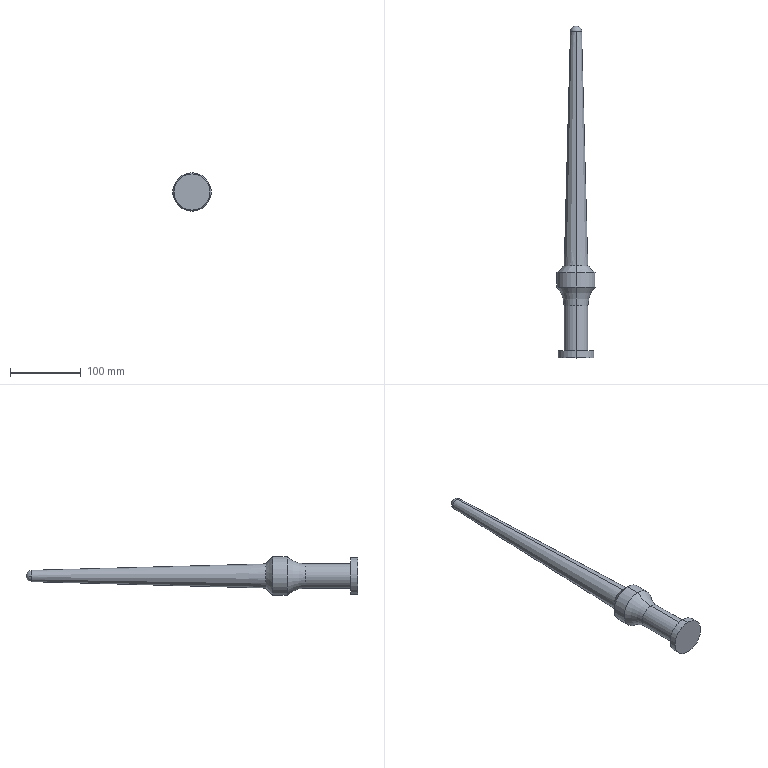Part | SolidWorks | features Revolution 1 | 1 solid | 16 faces | box 54 x 468 x 54 mm | volume 343926 mm3 | cylinder 6 | cone 4 | torus 2 | sphere 2 | plane 2 | commonest cylinder face diameters 34 x2 51 x2 54 x2
STEP:
#1=CARTESIAN_POINT('',(0.,0.,25.5));
#2=VERTEX_POINT('',#1);
#3=CARTESIAN_POINT('',(0.,0.,-25.5));
#4=VERTEX_POINT('',#3);
#5=CARTESIAN_POINT('',(0.,0.,0.));
#6=DIRECTION('',(0.,1.,0.));
#7=DIRECTION('',(0.,0.,1.));
#8=AXIS2_PLACEMENT_3D('',#5,#6,#7);
#9=CIRCLE('',#8,25.5);
#10=EDGE_CURVE('',#2,#4,#9,.T.);
#11=ORIENTED_EDGE('',*,*,#10,.T.);
#12=CARTESIAN_POINT('',(0.,10.,-25.5));
#13=VERTEX_POINT('',#12);
#14=CARTESIAN_POINT('',(0.,0.,-25.5));
#15=DIRECTION('',(0.,1.,0.));
#16=VECTOR('',#15,1000.);
#17=LINE('',#14,#16);
#18=EDGE_CURVE('',#4,#13,#17,.T.);
#19=ORIENTED_EDGE('',*,*,#18,.T.);
#20=CARTESIAN_POINT('',(0.,10.,25.5));
#21=VERTEX_POINT('',#20);
#22=CARTESIAN_POINT('',(0.,10.,0.));
#23=DIRECTION('',(0.,1.,0.));
#24=DIRECTION('',(0.,0.,1.));
#25=AXIS2_PLACEMENT_3D('',#22,#23,#24);
#26=CIRCLE('',#25,25.5);
#27=EDGE_CURVE('',#21,#13,#26,.T.);
#28=ORIENTED_EDGE('',*,*,#27,.F.);
#29=CARTESIAN_POINT('',(0.,0.,25.5));
#30=DIRECTION('',(0.,1.,0.));
#31=VECTOR('',#30,1000.);
#32=LINE('',#29,#31);
#33=EDGE_CURVE('',#2,#21,#32,.T.);
#34=ORIENTED_EDGE('',*,*,#33,.F.);
#35=EDGE_LOOP('',(#11,#19,#28,#34));
#36=FACE_OUTER_BOUND('',#35,.T.);
#37=CARTESIAN_POINT('',(0.,0.,0.));
#38=DIRECTION('',(0.,1.,0.));
#39=DIRECTION('',(0.,0.,1.));
#40=AXIS2_PLACEMENT_3D('',#37,#38,#39);
#41=CYLINDRICAL_SURFACE('',#40,25.5);
#42=ADVANCED_FACE('',(#36),#41,.T.);
#43=CARTESIAN_POINT('',(0.,10.,17.));
#44=VERTEX_POINT('',#43);
#45=CARTESIAN_POINT('',(0.,10.,-17.));
#46=VERTEX_POINT('',#45);
#47=CARTESIAN_POINT('',(0.,10.,0.));
#48=DIRECTION('',(0.,1.,0.));
#49=DIRECTION('',(0.,0.,1.));
#50=AXIS2_PLACEMENT_3D('',#47,#48,#49);
#51=CIRCLE('',#50,17.);
#52=EDGE_CURVE('',#44,#46,#51,.T.);
#53=ORIENTED_EDGE('',*,*,#52,.T.);
#54=CARTESIAN_POINT('',(0.,73.542,-17.));
#55=VERTEX_POINT('',#54);
#56=CARTESIAN_POINT('',(0.,0.,-17.));
#57=DIRECTION('',(0.,1.,0.));
#58=VECTOR('',#57,1000.);
#59=LINE('',#56,#58);
#60=EDGE_CURVE('',#46,#55,#59,.T.);
#61=ORIENTED_EDGE('',*,*,#60,.T.);
#62=CARTESIAN_POINT('',(0.,73.542,17.));
#63=VERTEX_POINT('',#62);
#64=CARTESIAN_POINT('',(0.,73.542,0.));
#65=DIRECTION('',(0.,1.,0.));
#66=DIRECTION('',(0.,0.,1.));
#67=AXIS2_PLACEMENT_3D('',#64,#65,#66);
#68=CIRCLE('',#67,17.);
#69=EDGE_CURVE('',#63,#55,#68,.T.);
#70=ORIENTED_EDGE('',*,*,#69,.F.);
#71=CARTESIAN_POINT('',(0.,0.,17.));
#72=DIRECTION('',(0.,1.,0.));
#73=VECTOR('',#72,1000.);
#74=LINE('',#71,#73);
#75=EDGE_CURVE('',#44,#63,#74,.T.);
#76=ORIENTED_EDGE('',*,*,#75,.F.);
#77=EDGE_LOOP('',(#53,#61,#70,#76));
#78=FACE_OUTER_BOUND('',#77,.T.);
#79=CARTESIAN_POINT('',(0.,0.,0.));
#80=DIRECTION('',(0.,1.,0.));
#81=DIRECTION('',(0.,0.,1.));
#82=AXIS2_PLACEMENT_3D('',#79,#80,#81);
#83=CYLINDRICAL_SURFACE('',#82,17.);
#84=ADVANCED_FACE('',(#78),#83,.T.);
#85=CARTESIAN_POINT('',(0.,100.,-27.));
#86=VERTEX_POINT('',#85);
#87=CARTESIAN_POINT('',(0.,100.,27.));
#88=VERTEX_POINT('',#87);
#89=CARTESIAN_POINT('',(0.,100.,0.));
#90=DIRECTION('',(0.,1.,0.));
#91=DIRECTION('',(0.,0.,1.));
#92=AXIS2_PLACEMENT_3D('',#89,#90,#91);
#93=CIRCLE('',#92,27.);
#94=EDGE_CURVE('',#86,#88,#93,.T.);
#95=ORIENTED_EDGE('',*,*,#94,.F.);
#96=CARTESIAN_POINT('',(0.,73.542,-57.));
#97=DIRECTION('',(1.,0.,0.));
#98=DIRECTION('',(0.,0.,-1.));
#99=AXIS2_PLACEMENT_3D('',#96,#97,#98);
#100=CIRCLE('',#99,40.);
#101=EDGE_CURVE('',#86,#55,#100,.T.);
#102=ORIENTED_EDGE('',*,*,#101,.T.);
#103=CARTESIAN_POINT('',(0.,73.542,0.));
#104=DIRECTION('',(0.,1.,0.));
#105=DIRECTION('',(0.,0.,1.));
#106=AXIS2_PLACEMENT_3D('',#103,#104,#105);
#107=CIRCLE('',#106,17.);
#108=EDGE_CURVE('',#55,#63,#107,.T.);
#109=ORIENTED_EDGE('',*,*,#108,.T.);
#110=CARTESIAN_POINT('',(0.,73.542,57.));
#111=DIRECTION('',(-1.,0.,0.));
#112=DIRECTION('',(0.,0.,1.));
#113=AXIS2_PLACEMENT_3D('',#110,#111,#112);
#114=CIRCLE('',#113,40.);
#115=EDGE_CURVE('',#88,#63,#114,.T.);
#116=ORIENTED_EDGE('',*,*,#115,.F.);
#117=EDGE_LOOP('',(#95,#102,#109,#116));
#118=FACE_OUTER_BOUND('',#117,.T.);
#119=CARTESIAN_POINT('',(0.,73.542,0.));
#120=DIRECTION('',(0.,1.,0.));
#121=DIRECTION('',(0.,0.,1.));
#122=AXIS2_PLACEMENT_3D('',#119,#120,#121);
#123=TOROIDAL_SURFACE('',#122,57.,40.);
#124=ADVANCED_FACE('',(#118),#123,.F.);
#125=CARTESIAN_POINT('',(0.,100.,0.));
#126=DIRECTION('',(0.,1.,0.));
#127=DIRECTION('',(0.,0.,1.));
#128=AXIS2_PLACEMENT_3D('',#125,#126,#127);
#129=CIRCLE('',#128,27.);
#130=EDGE_CURVE('',#88,#86,#129,.T.);
#131=ORIENTED_EDGE('',*,*,#130,.T.);
#132=CARTESIAN_POINT('',(0.,120.,-27.));
#133=VERTEX_POINT('',#132);
#134=CARTESIAN_POINT('',(0.,0.,-27.));
#135=DIRECTION('',(0.,1.,0.));
#136=VECTOR('',#135,1000.);
#137=LINE('',#134,#136);
#138=EDGE_CURVE('',#86,#133,#137,.T.);
#139=ORIENTED_EDGE('',*,*,#138,.T.);
#140=CARTESIAN_POINT('',(0.,120.,27.));
#141=VERTEX_POINT('',#140);
#142=CARTESIAN_POINT('',(0.,120.,0.));
#143=DIRECTION('',(0.,1.,0.));
#144=DIRECTION('',(0.,0.,1.));
#145=AXIS2_PLACEMENT_3D('',#142,#143,#144);
#146=CIRCLE('',#145,27.);
#147=EDGE_CURVE('',#141,#133,#146,.T.);
#148=ORIENTED_EDGE('',*,*,#147,.F.);
#149=CARTESIAN_POINT('',(0.,0.,27.));
#150=DIRECTION('',(0.,1.,0.));
#151=VECTOR('',#150,1000.);
#152=LINE('',#149,#151);
#153=EDGE_CURVE('',#88,#141,#152,.T.);
#154=ORIENTED_EDGE('',*,*,#153,.F.);
#155=EDGE_LOOP('',(#131,#139,#148,#154));
#156=FACE_OUTER_BOUND('',#155,.T.);
#157=CARTESIAN_POINT('',(0.,0.,0.));
#158=DIRECTION('',(0.,1.,0.));
#159=DIRECTION('',(0.,0.,1.));
#160=AXIS2_PLACEMENT_3D('',#157,#158,#159);
#161=CYLINDRICAL_SURFACE('',#160,27.);
#162=ADVANCED_FACE('',(#156),#161,.T.);
#163=CARTESIAN_POINT('',(0.,130.,17.));
#164=VERTEX_POINT('',#163);
#165=CARTESIAN_POINT('',(0.,130.,-17.));
#166=VERTEX_POINT('',#165);
#167=CARTESIAN_POINT('',(0.,130.,0.));
#168=DIRECTION('',(0.,1.,0.));
#169=DIRECTION('',(0.,0.,1.));
#170=AXIS2_PLACEMENT_3D('',#167,#168,#169);
#171=CIRCLE('',#170,17.);
#172=EDGE_CURVE('',#164,#166,#171,.T.);
#173=ORIENTED_EDGE('',*,*,#172,.F.);
#174=CARTESIAN_POINT('',(0.,120.,27.));
#175=DIRECTION('',(0.,-0.7071,0.7071));
#176=VECTOR('',#175,1000.);
#177=LINE('',#174,#176);
#178=EDGE_CURVE('',#164,#141,#177,.T.);
#179=ORIENTED_EDGE('',*,*,#178,.T.);
#180=ORIENTED_EDGE('',*,*,#147,.T.);
#181=CARTESIAN_POINT('',(0.,120.,-27.));
#182=DIRECTION('',(0.,-0.7071,-0.7071));
#183=VECTOR('',#182,1000.);
#184=LINE('',#181,#183);
#185=EDGE_CURVE('',#166,#133,#184,.T.);
#186=ORIENTED_EDGE('',*,*,#185,.F.);
#187=EDGE_LOOP('',(#173,#179,#180,#186));
#188=FACE_OUTER_BOUND('',#187,.T.);
#189=CARTESIAN_POINT('',(0.,120.,0.));
#190=DIRECTION('',(0.,-1.,0.));
#191=DIRECTION('',(0.,0.,-1.));
#192=AXIS2_PLACEMENT_3D('',#189,#190,#191);
#193=CONICAL_SURFACE('',#192,27.,0.7854);
#194=ADVANCED_FACE('',(#188),#193,.T.);
#195=CARTESIAN_POINT('',(0.,460.218,7.997));
#196=VERTEX_POINT('',#195);
#197=CARTESIAN_POINT('',(7.997,460.218,0.));
#198=VERTEX_POINT('',#197);
#199=CARTESIAN_POINT('',(0.,460.218,0.));
#200=DIRECTION('',(0.,1.,0.));
#201=DIRECTION('',(0.,0.,1.));
#202=AXIS2_PLACEMENT_3D('',#199,#200,#201);
#203=CIRCLE('',#202,7.997);
#204=EDGE_CURVE('',#196,#198,#203,.T.);
#205=ORIENTED_EDGE('',*,*,#204,.F.);
#206=CARTESIAN_POINT('',(0.,130.,17.));
#207=DIRECTION('',(0.,-0.9996,0.02725));
#208=VECTOR('',#207,1000.);
#209=LINE('',#206,#208);
#210=EDGE_CURVE('',#196,#164,#209,.T.);
#211=ORIENTED_EDGE('',*,*,#210,.T.);
#212=ORIENTED_EDGE('',*,*,#172,.T.);
#213=CARTESIAN_POINT('',(0.,460.218,-7.997));
#214=VERTEX_POINT('',#213);
#215=CARTESIAN_POINT('',(0.,130.,-17.));
#216=DIRECTION('',(0.,-0.9996,-0.02725));
#217=VECTOR('',#216,1000.);
#218=LINE('',#215,#217);
#219=EDGE_CURVE('',#214,#166,#218,.T.);
#220=ORIENTED_EDGE('',*,*,#219,.F.);
#221=CARTESIAN_POINT('',(0.,460.218,0.));
#222=DIRECTION('',(0.,1.,0.));
#223=DIRECTION('',(0.,0.,1.));
#224=AXIS2_PLACEMENT_3D('',#221,#222,#223);
#225=CIRCLE('',#224,7.997);
#226=EDGE_CURVE('',#198,#214,#225,.T.);
#227=ORIENTED_EDGE('',*,*,#226,.F.);
#228=EDGE_LOOP('',(#205,#211,#212,#220,#227));
#229=FACE_OUTER_BOUND('',#228,.T.);
#230=CARTESIAN_POINT('',(0.,130.,0.));
#231=DIRECTION('',(0.,-1.,0.));
#232=DIRECTION('',(0.,0.,-1.));
#233=AXIS2_PLACEMENT_3D('',#230,#231,#232);
#234=CONICAL_SURFACE('',#233,17.,0.02726);
#235=ADVANCED_FACE('',(#229),#234,.T.);
#236=ORIENTED_EDGE('',*,*,#226,.T.);
#237=CARTESIAN_POINT('',(-7.997,460.218,0.));
#238=VERTEX_POINT('',#237);
#239=CARTESIAN_POINT('',(0.,460.218,0.));
#240=DIRECTION('',(0.,1.,0.));
#241=DIRECTION('',(0.,0.,1.));
#242=AXIS2_PLACEMENT_3D('',#239,#240,#241);
#243=CIRCLE('',#242,7.997);
#244=EDGE_CURVE('',#214,#238,#243,.T.);
#245=ORIENTED_EDGE('',*,*,#244,.T.);
#246=CARTESIAN_POINT('',(0.,468.,0.));
#247=VERTEX_POINT('',#246);
#248=CARTESIAN_POINT('',(0.,460.,0.));
#249=DIRECTION('',(0.,0.,-1.));
#250=DIRECTION('',(-1.,0.,0.));
#251=AXIS2_PLACEMENT_3D('',#248,#249,#250);
#252=CIRCLE('',#251,8.);
#253=EDGE_CURVE('',#238,#247,#252,.T.);
#254=ORIENTED_EDGE('',*,*,#253,.T.);
#255=CARTESIAN_POINT('',(0.,460.,0.));
#256=DIRECTION('',(0.,0.,1.));
#257=DIRECTION('',(1.,0.,0.));
#258=AXIS2_PLACEMENT_3D('',#255,#256,#257);
#259=CIRCLE('',#258,8.);
#260=EDGE_CURVE('',#198,#247,#259,.T.);
#261=ORIENTED_EDGE('',*,*,#260,.F.);
#262=EDGE_LOOP('',(#236,#245,#254,#261));
#263=FACE_OUTER_BOUND('',#262,.T.);
#264=CARTESIAN_POINT('',(0.,460.,0.));
#265=DIRECTION('',(0.,0.,-1.));
#266=DIRECTION('',(1.,0.,0.));
#267=AXIS2_PLACEMENT_3D('',#264,#265,#266);
#268=SPHERICAL_SURFACE('',#267,8.);
#269=ADVANCED_FACE('',(#263),#268,.T.);
#270=ORIENTED_EDGE('',*,*,#253,.F.);
#271=CARTESIAN_POINT('',(0.,460.218,0.));
#272=DIRECTION('',(0.,1.,0.));
#273=DIRECTION('',(0.,0.,1.));
#274=AXIS2_PLACEMENT_3D('',#271,#272,#273);
#275=CIRCLE('',#274,7.997);
#276=EDGE_CURVE('',#238,#196,#275,.T.);
#277=ORIENTED_EDGE('',*,*,#276,.T.);
#278=ORIENTED_EDGE('',*,*,#204,.T.);
#279=ORIENTED_EDGE('',*,*,#260,.T.);
#280=EDGE_LOOP('',(#270,#277,#278,#279));
#281=FACE_OUTER_BOUND('',#280,.T.);
#282=CARTESIAN_POINT('',(0.,460.,0.));
#283=DIRECTION('',(0.,0.,-1.));
#284=DIRECTION('',(1.,0.,0.));
#285=AXIS2_PLACEMENT_3D('',#282,#283,#284);
#286=SPHERICAL_SURFACE('',#285,8.);
#287=ADVANCED_FACE('',(#281),#286,.T.);
#288=ORIENTED_EDGE('',*,*,#210,.F.);
#289=ORIENTED_EDGE('',*,*,#276,.F.);
#290=ORIENTED_EDGE('',*,*,#244,.F.);
#291=ORIENTED_EDGE('',*,*,#219,.T.);
#292=CARTESIAN_POINT('',(0.,130.,0.));
#293=DIRECTION('',(0.,1.,0.));
#294=DIRECTION('',(0.,0.,1.));
#295=AXIS2_PLACEMENT_3D('',#292,#293,#294);
#296=CIRCLE('',#295,17.);
#297=EDGE_CURVE('',#166,#164,#296,.T.);
#298=ORIENTED_EDGE('',*,*,#297,.T.);
#299=EDGE_LOOP('',(#288,#289,#290,#291,#298));
#300=FACE_OUTER_BOUND('',#299,.T.);
#301=CARTESIAN_POINT('',(0.,130.,0.));
#302=DIRECTION('',(0.,-1.,0.));
#303=DIRECTION('',(0.,0.,-1.));
#304=AXIS2_PLACEMENT_3D('',#301,#302,#303);
#305=CONICAL_SURFACE('',#304,17.,0.02726);
#306=ADVANCED_FACE('',(#300),#305,.T.);
#307=ORIENTED_EDGE('',*,*,#178,.F.);
#308=ORIENTED_EDGE('',*,*,#297,.F.);
#309=ORIENTED_EDGE('',*,*,#185,.T.);
#310=CARTESIAN_POINT('',(0.,120.,0.));
#311=DIRECTION('',(0.,1.,0.));
#312=DIRECTION('',(0.,0.,1.));
#313=AXIS2_PLACEMENT_3D('',#310,#311,#312);
#314=CIRCLE('',#313,27.);
#315=EDGE_CURVE('',#133,#141,#314,.T.);
#316=ORIENTED_EDGE('',*,*,#315,.T.);
#317=EDGE_LOOP('',(#307,#308,#309,#316));
#318=FACE_OUTER_BOUND('',#317,.T.);
#319=CARTESIAN_POINT('',(0.,120.,0.));
#320=DIRECTION('',(0.,-1.,0.));
#321=DIRECTION('',(0.,0.,-1.));
#322=AXIS2_PLACEMENT_3D('',#319,#320,#321);
#323=CONICAL_SURFACE('',#322,27.,0.7854);
#324=ADVANCED_FACE('',(#318),#323,.T.);
#325=ORIENTED_EDGE('',*,*,#138,.F.);
#326=ORIENTED_EDGE('',*,*,#94,.T.);
#327=ORIENTED_EDGE('',*,*,#153,.T.);
#328=ORIENTED_EDGE('',*,*,#315,.F.);
#329=EDGE_LOOP('',(#325,#326,#327,#328));
#330=FACE_OUTER_BOUND('',#329,.T.);
#331=CARTESIAN_POINT('',(0.,0.,0.));
#332=DIRECTION('',(0.,1.,0.));
#333=DIRECTION('',(0.,0.,1.));
#334=AXIS2_PLACEMENT_3D('',#331,#332,#333);
#335=CYLINDRICAL_SURFACE('',#334,27.);
#336=ADVANCED_FACE('',(#330),#335,.T.);
#337=ORIENTED_EDGE('',*,*,#101,.F.);
#338=ORIENTED_EDGE('',*,*,#130,.F.);
#339=ORIENTED_EDGE('',*,*,#115,.T.);
#340=ORIENTED_EDGE('',*,*,#69,.T.);
#341=EDGE_LOOP('',(#337,#338,#339,#340));
#342=FACE_OUTER_BOUND('',#341,.T.);
#343=CARTESIAN_POINT('',(0.,73.542,0.));
#344=DIRECTION('',(0.,1.,0.));
#345=DIRECTION('',(0.,0.,1.));
#346=AXIS2_PLACEMENT_3D('',#343,#344,#345);
#347=TOROIDAL_SURFACE('',#346,57.,40.);
#348=ADVANCED_FACE('',(#342),#347,.F.);
#349=ORIENTED_EDGE('',*,*,#60,.F.);
#350=CARTESIAN_POINT('',(0.,10.,0.));
#351=DIRECTION('',(0.,1.,0.));
#352=DIRECTION('',(0.,0.,1.));
#353=AXIS2_PLACEMENT_3D('',#350,#351,#352);
#354=CIRCLE('',#353,17.);
#355=EDGE_CURVE('',#46,#44,#354,.T.);
#356=ORIENTED_EDGE('',*,*,#355,.T.);
#357=ORIENTED_EDGE('',*,*,#75,.T.);
#358=ORIENTED_EDGE('',*,*,#108,.F.);
#359=EDGE_LOOP('',(#349,#356,#357,#358));
#360=FACE_OUTER_BOUND('',#359,.T.);
#361=CARTESIAN_POINT('',(0.,0.,0.));
#362=DIRECTION('',(0.,1.,0.));
#363=DIRECTION('',(0.,0.,1.));
#364=AXIS2_PLACEMENT_3D('',#361,#362,#363);
#365=CYLINDRICAL_SURFACE('',#364,17.);
#366=ADVANCED_FACE('',(#360),#365,.T.);
#367=ORIENTED_EDGE('',*,*,#52,.F.);
#368=ORIENTED_EDGE('',*,*,#355,.F.);
#369=EDGE_LOOP('',(#367,#368));
#370=FACE_BOUND('',#369,.T.);
#371=ORIENTED_EDGE('',*,*,#27,.T.);
#372=CARTESIAN_POINT('',(0.,10.,0.));
#373=DIRECTION('',(0.,1.,0.));
#374=DIRECTION('',(0.,0.,1.));
#375=AXIS2_PLACEMENT_3D('',#372,#373,#374);
#376=CIRCLE('',#375,25.5);
#377=EDGE_CURVE('',#13,#21,#376,.T.);
#378=ORIENTED_EDGE('',*,*,#377,.T.);
#379=EDGE_LOOP('',(#371,#378));
#380=FACE_OUTER_BOUND('',#379,.T.);
#381=CARTESIAN_POINT('',(25.5,10.,0.));
#382=DIRECTION('',(0.,-1.,0.));
#383=DIRECTION('',(0.,0.,-1.));
#384=AXIS2_PLACEMENT_3D('',#381,#382,#383);
#385=PLANE('',#384);
#386=ADVANCED_FACE('',(#370,#380),#385,.F.);
#387=ORIENTED_EDGE('',*,*,#18,.F.);
#388=CARTESIAN_POINT('',(0.,0.,0.));
#389=DIRECTION('',(0.,1.,0.));
#390=DIRECTION('',(0.,0.,1.));
#391=AXIS2_PLACEMENT_3D('',#388,#389,#390);
#392=CIRCLE('',#391,25.5);
#393=EDGE_CURVE('',#4,#2,#392,.T.);
#394=ORIENTED_EDGE('',*,*,#393,.T.);
#395=ORIENTED_EDGE('',*,*,#33,.T.);
#396=ORIENTED_EDGE('',*,*,#377,.F.);
#397=EDGE_LOOP('',(#387,#394,#395,#396));
#398=FACE_OUTER_BOUND('',#397,.T.);
#399=CARTESIAN_POINT('',(0.,0.,0.));
#400=DIRECTION('',(0.,1.,0.));
#401=DIRECTION('',(0.,0.,1.));
#402=AXIS2_PLACEMENT_3D('',#399,#400,#401);
#403=CYLINDRICAL_SURFACE('',#402,25.5);
#404=ADVANCED_FACE('',(#398),#403,.T.);
#405=ORIENTED_EDGE('',*,*,#10,.F.);
#406=ORIENTED_EDGE('',*,*,#393,.F.);
#407=EDGE_LOOP('',(#405,#406));
#408=FACE_OUTER_BOUND('',#407,.T.);
#409=CARTESIAN_POINT('',(0.,0.,0.));
#410=DIRECTION('',(0.,1.,0.));
#411=DIRECTION('',(0.,0.,1.));
#412=AXIS2_PLACEMENT_3D('',#409,#410,#411);
#413=PLANE('',#412);
#414=ADVANCED_FACE('',(#408),#413,.F.);
#415=CLOSED_SHELL('',(#42,#84,#124,#162,#194,#235,#269,#287,#306,#324,#336,#348,#366,#386,#404,#414));
#416=MANIFOLD_SOLID_BREP('',#415);
#417=CARTESIAN_POINT('',(0.,0.,0.));
#418=DIRECTION('',(0.,0.,1.));
#419=DIRECTION('',(1.,0.,0.));
#420=AXIS2_PLACEMENT_3D('',#417,#418,#419);
#421=(LENGTH_UNIT()NAMED_UNIT(*)SI_UNIT(.MILLI.,.METRE.));
#422=UNCERTAINTY_MEASURE_WITH_UNIT(LENGTH_MEASURE(0.00001),#421,'','');
#423=(NAMED_UNIT(*)PLANE_ANGLE_UNIT()SI_UNIT($,.RADIAN.));
#424=(NAMED_UNIT(*)SI_UNIT($,.STERADIAN.)SOLID_ANGLE_UNIT());
#425=(GEOMETRIC_REPRESENTATION_CONTEXT(3)GLOBAL_UNCERTAINTY_ASSIGNED_CONTEXT((#422))GLOBAL_UNIT_ASSIGNED_CONTEXT((#421,#423,#424))REPRESENTATION_CONTEXT('',''));
#426=ADVANCED_BREP_SHAPE_REPRESENTATION('',(#416,#420),#425);